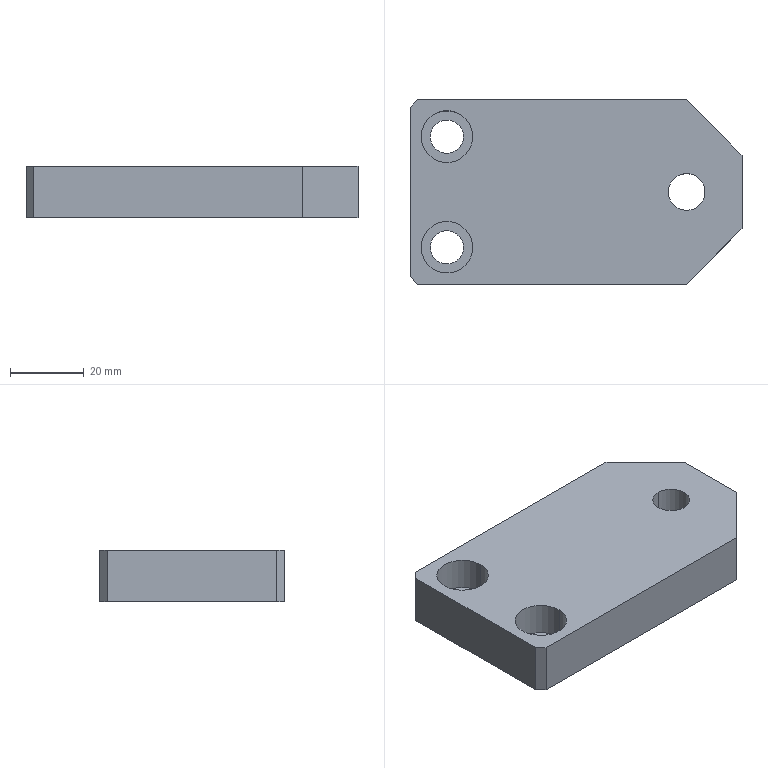Part | STEP file | J454-EBZ05-29-00-Part-1 | 1 solid | 22 faces | box 90 x 50 x 14 mm | volume 55287 mm3 | plane 12 | cylinder 10 | commonest cylinder face diameters 9 x4 14 x4 10 x2
STEP:
#1=CARTESIAN_POINT('',(14.5,40.,-2.));
#2=VERTEX_POINT('',#1);
#3=CARTESIAN_POINT('',(5.5,40.,-2.));
#4=VERTEX_POINT('',#3);
#5=CARTESIAN_POINT('',(10.,40.,-2.));
#6=DIRECTION('',(0.,0.,1.));
#7=DIRECTION('',(-1.,0.,0.));
#8=AXIS2_PLACEMENT_3D('',#5,#6,#7);
#9=CIRCLE('',#8,4.5);
#10=EDGE_CURVE('',#2,#4,#9,.T.);
#11=ORIENTED_EDGE('',*,*,#10,.F.);
#12=CARTESIAN_POINT('',(14.5,40.,3.));
#13=VERTEX_POINT('',#12);
#14=CARTESIAN_POINT('',(14.5,40.,12.));
#15=DIRECTION('',(0.,0.,1.));
#16=VECTOR('',#15,1000.);
#17=LINE('',#14,#16);
#18=EDGE_CURVE('',#2,#13,#17,.T.);
#19=ORIENTED_EDGE('',*,*,#18,.T.);
#20=CARTESIAN_POINT('',(5.5,40.,3.));
#21=VERTEX_POINT('',#20);
#22=CARTESIAN_POINT('',(10.,40.,3.));
#23=DIRECTION('',(0.,0.,1.));
#24=DIRECTION('',(-1.,0.,0.));
#25=AXIS2_PLACEMENT_3D('',#22,#23,#24);
#26=CIRCLE('',#25,4.5);
#27=EDGE_CURVE('',#13,#21,#26,.T.);
#28=ORIENTED_EDGE('',*,*,#27,.T.);
#29=CARTESIAN_POINT('',(5.5,40.,12.));
#30=DIRECTION('',(0.,0.,1.));
#31=VECTOR('',#30,1000.);
#32=LINE('',#29,#31);
#33=EDGE_CURVE('',#4,#21,#32,.T.);
#34=ORIENTED_EDGE('',*,*,#33,.F.);
#35=EDGE_LOOP('',(#11,#19,#28,#34));
#36=FACE_OUTER_BOUND('',#35,.T.);
#37=CARTESIAN_POINT('',(10.,40.,12.));
#38=DIRECTION('',(0.,0.,1.));
#39=DIRECTION('',(-1.,0.,0.));
#40=AXIS2_PLACEMENT_3D('',#37,#38,#39);
#41=CYLINDRICAL_SURFACE('',#40,4.5);
#42=ADVANCED_FACE('',(#36),#41,.F.);
#43=CARTESIAN_POINT('',(17.,40.,3.));
#44=VERTEX_POINT('',#43);
#45=CARTESIAN_POINT('',(3.,40.,3.));
#46=VERTEX_POINT('',#45);
#47=CARTESIAN_POINT('',(10.,40.,3.));
#48=DIRECTION('',(0.,0.,1.));
#49=DIRECTION('',(-1.,0.,0.));
#50=AXIS2_PLACEMENT_3D('',#47,#48,#49);
#51=CIRCLE('',#50,7.);
#52=EDGE_CURVE('',#44,#46,#51,.T.);
#53=ORIENTED_EDGE('',*,*,#52,.F.);
#54=CARTESIAN_POINT('',(17.,40.,12.));
#55=VERTEX_POINT('',#54);
#56=CARTESIAN_POINT('',(17.,40.,12.));
#57=DIRECTION('',(0.,0.,1.));
#58=VECTOR('',#57,1000.);
#59=LINE('',#56,#58);
#60=EDGE_CURVE('',#44,#55,#59,.T.);
#61=ORIENTED_EDGE('',*,*,#60,.T.);
#62=CARTESIAN_POINT('',(3.,40.,12.));
#63=VERTEX_POINT('',#62);
#64=CARTESIAN_POINT('',(10.,40.,12.));
#65=DIRECTION('',(0.,0.,1.));
#66=DIRECTION('',(-1.,0.,0.));
#67=AXIS2_PLACEMENT_3D('',#64,#65,#66);
#68=CIRCLE('',#67,7.);
#69=EDGE_CURVE('',#55,#63,#68,.T.);
#70=ORIENTED_EDGE('',*,*,#69,.T.);
#71=CARTESIAN_POINT('',(3.,40.,12.));
#72=DIRECTION('',(0.,0.,1.));
#73=VECTOR('',#72,1000.);
#74=LINE('',#71,#73);
#75=EDGE_CURVE('',#46,#63,#74,.T.);
#76=ORIENTED_EDGE('',*,*,#75,.F.);
#77=EDGE_LOOP('',(#53,#61,#70,#76));
#78=FACE_OUTER_BOUND('',#77,.T.);
#79=CARTESIAN_POINT('',(10.,40.,12.));
#80=DIRECTION('',(0.,0.,1.));
#81=DIRECTION('',(-1.,0.,0.));
#82=AXIS2_PLACEMENT_3D('',#79,#80,#81);
#83=CYLINDRICAL_SURFACE('',#82,7.);
#84=ADVANCED_FACE('',(#78),#83,.F.);
#85=CARTESIAN_POINT('',(14.5,10.,-2.));
#86=VERTEX_POINT('',#85);
#87=CARTESIAN_POINT('',(5.5,10.,-2.));
#88=VERTEX_POINT('',#87);
#89=CARTESIAN_POINT('',(10.,10.,-2.));
#90=DIRECTION('',(0.,0.,1.));
#91=DIRECTION('',(-1.,0.,0.));
#92=AXIS2_PLACEMENT_3D('',#89,#90,#91);
#93=CIRCLE('',#92,4.5);
#94=EDGE_CURVE('',#86,#88,#93,.T.);
#95=ORIENTED_EDGE('',*,*,#94,.F.);
#96=CARTESIAN_POINT('',(14.5,10.,3.));
#97=VERTEX_POINT('',#96);
#98=CARTESIAN_POINT('',(14.5,10.,12.));
#99=DIRECTION('',(0.,0.,1.));
#100=VECTOR('',#99,1000.);
#101=LINE('',#98,#100);
#102=EDGE_CURVE('',#86,#97,#101,.T.);
#103=ORIENTED_EDGE('',*,*,#102,.T.);
#104=CARTESIAN_POINT('',(5.5,10.,3.));
#105=VERTEX_POINT('',#104);
#106=CARTESIAN_POINT('',(10.,10.,3.));
#107=DIRECTION('',(0.,0.,1.));
#108=DIRECTION('',(-1.,0.,0.));
#109=AXIS2_PLACEMENT_3D('',#106,#107,#108);
#110=CIRCLE('',#109,4.5);
#111=EDGE_CURVE('',#97,#105,#110,.T.);
#112=ORIENTED_EDGE('',*,*,#111,.T.);
#113=CARTESIAN_POINT('',(5.5,10.,12.));
#114=DIRECTION('',(0.,0.,1.));
#115=VECTOR('',#114,1000.);
#116=LINE('',#113,#115);
#117=EDGE_CURVE('',#88,#105,#116,.T.);
#118=ORIENTED_EDGE('',*,*,#117,.F.);
#119=EDGE_LOOP('',(#95,#103,#112,#118));
#120=FACE_OUTER_BOUND('',#119,.T.);
#121=CARTESIAN_POINT('',(10.,10.,12.));
#122=DIRECTION('',(0.,0.,1.));
#123=DIRECTION('',(-1.,0.,0.));
#124=AXIS2_PLACEMENT_3D('',#121,#122,#123);
#125=CYLINDRICAL_SURFACE('',#124,4.5);
#126=ADVANCED_FACE('',(#120),#125,.F.);
#127=CARTESIAN_POINT('',(17.,10.,3.));
#128=VERTEX_POINT('',#127);
#129=CARTESIAN_POINT('',(3.,10.,3.));
#130=VERTEX_POINT('',#129);
#131=CARTESIAN_POINT('',(10.,10.,3.));
#132=DIRECTION('',(0.,0.,1.));
#133=DIRECTION('',(-1.,0.,0.));
#134=AXIS2_PLACEMENT_3D('',#131,#132,#133);
#135=CIRCLE('',#134,7.);
#136=EDGE_CURVE('',#128,#130,#135,.T.);
#137=ORIENTED_EDGE('',*,*,#136,.F.);
#138=CARTESIAN_POINT('',(17.,10.,12.));
#139=VERTEX_POINT('',#138);
#140=CARTESIAN_POINT('',(17.,10.,12.));
#141=DIRECTION('',(0.,0.,1.));
#142=VECTOR('',#141,1000.);
#143=LINE('',#140,#142);
#144=EDGE_CURVE('',#128,#139,#143,.T.);
#145=ORIENTED_EDGE('',*,*,#144,.T.);
#146=CARTESIAN_POINT('',(3.,10.,12.));
#147=VERTEX_POINT('',#146);
#148=CARTESIAN_POINT('',(10.,10.,12.));
#149=DIRECTION('',(0.,0.,1.));
#150=DIRECTION('',(-1.,0.,0.));
#151=AXIS2_PLACEMENT_3D('',#148,#149,#150);
#152=CIRCLE('',#151,7.);
#153=EDGE_CURVE('',#139,#147,#152,.T.);
#154=ORIENTED_EDGE('',*,*,#153,.T.);
#155=CARTESIAN_POINT('',(3.,10.,12.));
#156=DIRECTION('',(0.,0.,1.));
#157=VECTOR('',#156,1000.);
#158=LINE('',#155,#157);
#159=EDGE_CURVE('',#130,#147,#158,.T.);
#160=ORIENTED_EDGE('',*,*,#159,.F.);
#161=EDGE_LOOP('',(#137,#145,#154,#160));
#162=FACE_OUTER_BOUND('',#161,.T.);
#163=CARTESIAN_POINT('',(10.,10.,12.));
#164=DIRECTION('',(0.,0.,1.));
#165=DIRECTION('',(-1.,0.,0.));
#166=AXIS2_PLACEMENT_3D('',#163,#164,#165);
#167=CYLINDRICAL_SURFACE('',#166,7.);
#168=ADVANCED_FACE('',(#162),#167,.F.);
#169=CARTESIAN_POINT('',(75.,30.,12.));
#170=VERTEX_POINT('',#169);
#171=CARTESIAN_POINT('',(75.,20.,12.));
#172=VERTEX_POINT('',#171);
#173=CARTESIAN_POINT('',(75.,25.,12.));
#174=DIRECTION('',(0.,0.,-1.));
#175=DIRECTION('',(0.,-1.,0.));
#176=AXIS2_PLACEMENT_3D('',#173,#174,#175);
#177=CIRCLE('',#176,5.);
#178=EDGE_CURVE('',#170,#172,#177,.T.);
#179=ORIENTED_EDGE('',*,*,#178,.F.);
#180=CARTESIAN_POINT('',(75.,30.,-2.));
#181=VERTEX_POINT('',#180);
#182=CARTESIAN_POINT('',(75.,30.,12.));
#183=DIRECTION('',(0.,0.,-1.));
#184=VECTOR('',#183,1000.);
#185=LINE('',#182,#184);
#186=EDGE_CURVE('',#170,#181,#185,.T.);
#187=ORIENTED_EDGE('',*,*,#186,.T.);
#188=CARTESIAN_POINT('',(75.,20.,-2.));
#189=VERTEX_POINT('',#188);
#190=CARTESIAN_POINT('',(75.,25.,-2.));
#191=DIRECTION('',(0.,0.,1.));
#192=DIRECTION('',(0.,1.,0.));
#193=AXIS2_PLACEMENT_3D('',#190,#191,#192);
#194=CIRCLE('',#193,5.);
#195=EDGE_CURVE('',#189,#181,#194,.T.);
#196=ORIENTED_EDGE('',*,*,#195,.F.);
#197=CARTESIAN_POINT('',(75.,20.,12.));
#198=DIRECTION('',(0.,0.,-1.));
#199=VECTOR('',#198,1000.);
#200=LINE('',#197,#199);
#201=EDGE_CURVE('',#172,#189,#200,.T.);
#202=ORIENTED_EDGE('',*,*,#201,.F.);
#203=EDGE_LOOP('',(#179,#187,#196,#202));
#204=FACE_OUTER_BOUND('',#203,.T.);
#205=CARTESIAN_POINT('',(75.,25.,12.));
#206=DIRECTION('',(0.,0.,-1.));
#207=DIRECTION('',(0.,-1.,0.));
#208=AXIS2_PLACEMENT_3D('',#205,#206,#207);
#209=CYLINDRICAL_SURFACE('',#208,5.);
#210=ADVANCED_FACE('',(#204),#209,.F.);
#211=CARTESIAN_POINT('',(10.,40.,12.));
#212=DIRECTION('',(0.,0.,1.));
#213=DIRECTION('',(-1.,0.,0.));
#214=AXIS2_PLACEMENT_3D('',#211,#212,#213);
#215=CIRCLE('',#214,7.);
#216=EDGE_CURVE('',#63,#55,#215,.T.);
#217=ORIENTED_EDGE('',*,*,#216,.F.);
#218=ORIENTED_EDGE('',*,*,#69,.F.);
#219=EDGE_LOOP('',(#217,#218));
#220=FACE_BOUND('',#219,.T.);
#221=CARTESIAN_POINT('',(10.,10.,12.));
#222=DIRECTION('',(0.,0.,1.));
#223=DIRECTION('',(-1.,0.,0.));
#224=AXIS2_PLACEMENT_3D('',#221,#222,#223);
#225=CIRCLE('',#224,7.);
#226=EDGE_CURVE('',#147,#139,#225,.T.);
#227=ORIENTED_EDGE('',*,*,#226,.F.);
#228=ORIENTED_EDGE('',*,*,#153,.F.);
#229=EDGE_LOOP('',(#227,#228));
#230=FACE_BOUND('',#229,.T.);
#231=CARTESIAN_POINT('',(75.,25.,12.));
#232=DIRECTION('',(0.,0.,-1.));
#233=DIRECTION('',(0.,-1.,0.));
#234=AXIS2_PLACEMENT_3D('',#231,#232,#233);
#235=CIRCLE('',#234,5.);
#236=EDGE_CURVE('',#172,#170,#235,.T.);
#237=ORIENTED_EDGE('',*,*,#236,.T.);
#238=ORIENTED_EDGE('',*,*,#178,.T.);
#239=EDGE_LOOP('',(#237,#238));
#240=FACE_BOUND('',#239,.T.);
#241=CARTESIAN_POINT('',(2.,50.,12.));
#242=VERTEX_POINT('',#241);
#243=CARTESIAN_POINT('',(75.,50.,12.));
#244=VERTEX_POINT('',#243);
#245=CARTESIAN_POINT('',(45.,50.,12.));
#246=DIRECTION('',(1.,0.,0.));
#247=VECTOR('',#246,1000.);
#248=LINE('',#245,#247);
#249=EDGE_CURVE('',#242,#244,#248,.T.);
#250=ORIENTED_EDGE('',*,*,#249,.F.);
#251=CARTESIAN_POINT('',(0.,48.,12.));
#252=VERTEX_POINT('',#251);
#253=CARTESIAN_POINT('',(11.,59.,12.));
#254=DIRECTION('',(-0.7071,-0.7071,0.));
#255=VECTOR('',#254,1000.);
#256=LINE('',#253,#255);
#257=EDGE_CURVE('',#242,#252,#256,.T.);
#258=ORIENTED_EDGE('',*,*,#257,.T.);
#259=CARTESIAN_POINT('',(0.,2.,12.));
#260=VERTEX_POINT('',#259);
#261=CARTESIAN_POINT('',(0.,25.,12.));
#262=DIRECTION('',(0.,1.,0.));
#263=VECTOR('',#262,1000.);
#264=LINE('',#261,#263);
#265=EDGE_CURVE('',#260,#252,#264,.T.);
#266=ORIENTED_EDGE('',*,*,#265,.F.);
#267=CARTESIAN_POINT('',(2.,0.,12.));
#268=VERTEX_POINT('',#267);
#269=CARTESIAN_POINT('',(11.,-9.,12.));
#270=DIRECTION('',(0.7071,-0.7071,0.));
#271=VECTOR('',#270,1000.);
#272=LINE('',#269,#271);
#273=EDGE_CURVE('',#260,#268,#272,.T.);
#274=ORIENTED_EDGE('',*,*,#273,.T.);
#275=CARTESIAN_POINT('',(75.,0.,12.));
#276=VERTEX_POINT('',#275);
#277=CARTESIAN_POINT('',(45.,0.,12.));
#278=DIRECTION('',(-1.,0.,0.));
#279=VECTOR('',#278,1000.);
#280=LINE('',#277,#279);
#281=EDGE_CURVE('',#276,#268,#280,.T.);
#282=ORIENTED_EDGE('',*,*,#281,.F.);
#283=CARTESIAN_POINT('',(90.,15.,12.));
#284=VERTEX_POINT('',#283);
#285=CARTESIAN_POINT('',(72.5,-2.5,12.));
#286=DIRECTION('',(0.7071,0.7071,0.));
#287=VECTOR('',#286,1000.);
#288=LINE('',#285,#287);
#289=EDGE_CURVE('',#276,#284,#288,.T.);
#290=ORIENTED_EDGE('',*,*,#289,.T.);
#291=CARTESIAN_POINT('',(90.,35.,12.));
#292=VERTEX_POINT('',#291);
#293=CARTESIAN_POINT('',(90.,25.,12.));
#294=DIRECTION('',(0.,-1.,0.));
#295=VECTOR('',#294,1000.);
#296=LINE('',#293,#295);
#297=EDGE_CURVE('',#292,#284,#296,.T.);
#298=ORIENTED_EDGE('',*,*,#297,.F.);
#299=CARTESIAN_POINT('',(72.5,52.5,12.));
#300=DIRECTION('',(-0.7071,0.7071,0.));
#301=VECTOR('',#300,1000.);
#302=LINE('',#299,#301);
#303=EDGE_CURVE('',#292,#244,#302,.T.);
#304=ORIENTED_EDGE('',*,*,#303,.T.);
#305=EDGE_LOOP('',(#250,#258,#266,#274,#282,#290,#298,#304));
#306=FACE_OUTER_BOUND('',#305,.T.);
#307=CARTESIAN_POINT('',(45.,25.,12.));
#308=DIRECTION('',(0.,0.,1.));
#309=DIRECTION('',(0.,1.,0.));
#310=AXIS2_PLACEMENT_3D('',#307,#308,#309);
#311=PLANE('',#310);
#312=ADVANCED_FACE('',(#220,#230,#240,#306),#311,.T.);
#313=CARTESIAN_POINT('',(90.,15.,-2.));
#314=VERTEX_POINT('',#313);
#315=CARTESIAN_POINT('',(90.,35.,-2.));
#316=VERTEX_POINT('',#315);
#317=CARTESIAN_POINT('',(90.,25.,-2.));
#318=DIRECTION('',(0.,1.,0.));
#319=VECTOR('',#318,1000.);
#320=LINE('',#317,#319);
#321=EDGE_CURVE('',#314,#316,#320,.T.);
#322=ORIENTED_EDGE('',*,*,#321,.T.);
#323=CARTESIAN_POINT('',(90.,35.,-2.));
#324=DIRECTION('',(0.,0.,1.));
#325=VECTOR('',#324,1000.);
#326=LINE('',#323,#325);
#327=EDGE_CURVE('',#316,#292,#326,.T.);
#328=ORIENTED_EDGE('',*,*,#327,.T.);
#329=ORIENTED_EDGE('',*,*,#297,.T.);
#330=CARTESIAN_POINT('',(90.,15.,-2.));
#331=DIRECTION('',(0.,0.,-1.));
#332=VECTOR('',#331,1000.);
#333=LINE('',#330,#332);
#334=EDGE_CURVE('',#284,#314,#333,.T.);
#335=ORIENTED_EDGE('',*,*,#334,.T.);
#336=EDGE_LOOP('',(#322,#328,#329,#335));
#337=FACE_OUTER_BOUND('',#336,.T.);
#338=CARTESIAN_POINT('',(90.,25.,-2.));
#339=DIRECTION('',(1.,0.,0.));
#340=DIRECTION('',(0.,0.,-1.));
#341=AXIS2_PLACEMENT_3D('',#338,#339,#340);
#342=PLANE('',#341);
#343=ADVANCED_FACE('',(#337),#342,.T.);
#344=ORIENTED_EDGE('',*,*,#281,.T.);
#345=CARTESIAN_POINT('',(2.,0.,-2.));
#346=VERTEX_POINT('',#345);
#347=CARTESIAN_POINT('',(2.,0.,-2.));
#348=DIRECTION('',(0.,0.,-1.));
#349=VECTOR('',#348,1000.);
#350=LINE('',#347,#349);
#351=EDGE_CURVE('',#268,#346,#350,.T.);
#352=ORIENTED_EDGE('',*,*,#351,.T.);
#353=CARTESIAN_POINT('',(75.,0.,-2.));
#354=VERTEX_POINT('',#353);
#355=CARTESIAN_POINT('',(45.,0.,-2.));
#356=DIRECTION('',(1.,0.,0.));
#357=VECTOR('',#356,1000.);
#358=LINE('',#355,#357);
#359=EDGE_CURVE('',#346,#354,#358,.T.);
#360=ORIENTED_EDGE('',*,*,#359,.T.);
#361=CARTESIAN_POINT('',(75.,0.,-2.));
#362=DIRECTION('',(0.,0.,1.));
#363=VECTOR('',#362,1000.);
#364=LINE('',#361,#363);
#365=EDGE_CURVE('',#354,#276,#364,.T.);
#366=ORIENTED_EDGE('',*,*,#365,.T.);
#367=EDGE_LOOP('',(#344,#352,#360,#366));
#368=FACE_OUTER_BOUND('',#367,.T.);
#369=CARTESIAN_POINT('',(45.,0.,-2.));
#370=DIRECTION('',(0.,-1.,0.));
#371=DIRECTION('',(0.,0.,1.));
#372=AXIS2_PLACEMENT_3D('',#369,#370,#371);
#373=PLANE('',#372);
#374=ADVANCED_FACE('',(#368),#373,.T.);
#375=ORIENTED_EDGE('',*,*,#265,.T.);
#376=CARTESIAN_POINT('',(0.,48.,-2.));
#377=VERTEX_POINT('',#376);
#378=CARTESIAN_POINT('',(0.,48.,-2.));
#379=DIRECTION('',(0.,0.,-1.));
#380=VECTOR('',#379,1000.);
#381=LINE('',#378,#380);
#382=EDGE_CURVE('',#252,#377,#381,.T.);
#383=ORIENTED_EDGE('',*,*,#382,.T.);
#384=CARTESIAN_POINT('',(0.,2.,-2.));
#385=VERTEX_POINT('',#384);
#386=CARTESIAN_POINT('',(0.,25.,-2.));
#387=DIRECTION('',(0.,-1.,0.));
#388=VECTOR('',#387,1000.);
#389=LINE('',#386,#388);
#390=EDGE_CURVE('',#377,#385,#389,.T.);
#391=ORIENTED_EDGE('',*,*,#390,.T.);
#392=CARTESIAN_POINT('',(0.,2.,-2.));
#393=DIRECTION('',(0.,0.,1.));
#394=VECTOR('',#393,1000.);
#395=LINE('',#392,#394);
#396=EDGE_CURVE('',#385,#260,#395,.T.);
#397=ORIENTED_EDGE('',*,*,#396,.T.);
#398=EDGE_LOOP('',(#375,#383,#391,#397));
#399=FACE_OUTER_BOUND('',#398,.T.);
#400=CARTESIAN_POINT('',(0.,25.,-2.));
#401=DIRECTION('',(-1.,0.,0.));
#402=DIRECTION('',(0.,0.,1.));
#403=AXIS2_PLACEMENT_3D('',#400,#401,#402);
#404=PLANE('',#403);
#405=ADVANCED_FACE('',(#399),#404,.T.);
#406=CARTESIAN_POINT('',(10.,40.,-2.));
#407=DIRECTION('',(0.,0.,1.));
#408=DIRECTION('',(-1.,0.,0.));
#409=AXIS2_PLACEMENT_3D('',#406,#407,#408);
#410=CIRCLE('',#409,4.5);
#411=EDGE_CURVE('',#4,#2,#410,.T.);
#412=ORIENTED_EDGE('',*,*,#411,.T.);
#413=ORIENTED_EDGE('',*,*,#10,.T.);
#414=EDGE_LOOP('',(#412,#413));
#415=FACE_BOUND('',#414,.T.);
#416=CARTESIAN_POINT('',(10.,10.,-2.));
#417=DIRECTION('',(0.,0.,1.));
#418=DIRECTION('',(-1.,0.,0.));
#419=AXIS2_PLACEMENT_3D('',#416,#417,#418);
#420=CIRCLE('',#419,4.5);
#421=EDGE_CURVE('',#88,#86,#420,.T.);
#422=ORIENTED_EDGE('',*,*,#421,.T.);
#423=ORIENTED_EDGE('',*,*,#94,.T.);
#424=EDGE_LOOP('',(#422,#423));
#425=FACE_BOUND('',#424,.T.);
#426=ORIENTED_EDGE('',*,*,#195,.T.);
#427=CARTESIAN_POINT('',(75.,25.,-2.));
#428=DIRECTION('',(0.,0.,1.));
#429=DIRECTION('',(0.,1.,0.));
#430=AXIS2_PLACEMENT_3D('',#427,#428,#429);
#431=CIRCLE('',#430,5.);
#432=EDGE_CURVE('',#181,#189,#431,.T.);
#433=ORIENTED_EDGE('',*,*,#432,.T.);
#434=EDGE_LOOP('',(#426,#433));
#435=FACE_BOUND('',#434,.T.);
#436=ORIENTED_EDGE('',*,*,#390,.F.);
#437=CARTESIAN_POINT('',(2.,50.,-2.));
#438=VERTEX_POINT('',#437);
#439=CARTESIAN_POINT('',(11.,59.,-2.));
#440=DIRECTION('',(0.7071,0.7071,0.));
#441=VECTOR('',#440,1000.);
#442=LINE('',#439,#441);
#443=EDGE_CURVE('',#377,#438,#442,.T.);
#444=ORIENTED_EDGE('',*,*,#443,.T.);
#445=CARTESIAN_POINT('',(75.,50.,-2.));
#446=VERTEX_POINT('',#445);
#447=CARTESIAN_POINT('',(45.,50.,-2.));
#448=DIRECTION('',(-1.,0.,0.));
#449=VECTOR('',#448,1000.);
#450=LINE('',#447,#449);
#451=EDGE_CURVE('',#446,#438,#450,.T.);
#452=ORIENTED_EDGE('',*,*,#451,.F.);
#453=CARTESIAN_POINT('',(72.5,52.5,-2.));
#454=DIRECTION('',(0.7071,-0.7071,0.));
#455=VECTOR('',#454,1000.);
#456=LINE('',#453,#455);
#457=EDGE_CURVE('',#446,#316,#456,.T.);
#458=ORIENTED_EDGE('',*,*,#457,.T.);
#459=ORIENTED_EDGE('',*,*,#321,.F.);
#460=CARTESIAN_POINT('',(72.5,-2.5,-2.));
#461=DIRECTION('',(-0.7071,-0.7071,0.));
#462=VECTOR('',#461,1000.);
#463=LINE('',#460,#462);
#464=EDGE_CURVE('',#314,#354,#463,.T.);
#465=ORIENTED_EDGE('',*,*,#464,.T.);
#466=ORIENTED_EDGE('',*,*,#359,.F.);
#467=CARTESIAN_POINT('',(11.,-9.,-2.));
#468=DIRECTION('',(-0.7071,0.7071,0.));
#469=VECTOR('',#468,1000.);
#470=LINE('',#467,#469);
#471=EDGE_CURVE('',#346,#385,#470,.T.);
#472=ORIENTED_EDGE('',*,*,#471,.T.);
#473=EDGE_LOOP('',(#436,#444,#452,#458,#459,#465,#466,#472));
#474=FACE_OUTER_BOUND('',#473,.T.);
#475=CARTESIAN_POINT('',(45.,25.,-2.));
#476=DIRECTION('',(0.,0.,-1.));
#477=DIRECTION('',(0.,-1.,0.));
#478=AXIS2_PLACEMENT_3D('',#475,#476,#477);
#479=PLANE('',#478);
#480=ADVANCED_FACE('',(#415,#425,#435,#474),#479,.T.);
#481=ORIENTED_EDGE('',*,*,#451,.T.);
#482=CARTESIAN_POINT('',(2.,50.,-2.));
#483=DIRECTION('',(0.,0.,1.));
#484=VECTOR('',#483,1000.);
#485=LINE('',#482,#484);
#486=EDGE_CURVE('',#438,#242,#485,.T.);
#487=ORIENTED_EDGE('',*,*,#486,.T.);
#488=ORIENTED_EDGE('',*,*,#249,.T.);
#489=CARTESIAN_POINT('',(75.,50.,-2.));
#490=DIRECTION('',(0.,0.,-1.));
#491=VECTOR('',#490,1000.);
#492=LINE('',#489,#491);
#493=EDGE_CURVE('',#244,#446,#492,.T.);
#494=ORIENTED_EDGE('',*,*,#493,.T.);
#495=EDGE_LOOP('',(#481,#487,#488,#494));
#496=FACE_OUTER_BOUND('',#495,.T.);
#497=CARTESIAN_POINT('',(45.,50.,-2.));
#498=DIRECTION('',(0.,1.,0.));
#499=DIRECTION('',(0.,0.,-1.));
#500=AXIS2_PLACEMENT_3D('',#497,#498,#499);
#501=PLANE('',#500);
#502=ADVANCED_FACE('',(#496),#501,.T.);
#503=ORIENTED_EDGE('',*,*,#186,.F.);
#504=ORIENTED_EDGE('',*,*,#236,.F.);
#505=ORIENTED_EDGE('',*,*,#201,.T.);
#506=ORIENTED_EDGE('',*,*,#432,.F.);
#507=EDGE_LOOP('',(#503,#504,#505,#506));
#508=FACE_OUTER_BOUND('',#507,.T.);
#509=CARTESIAN_POINT('',(75.,25.,12.));
#510=DIRECTION('',(0.,0.,-1.));
#511=DIRECTION('',(0.,-1.,0.));
#512=AXIS2_PLACEMENT_3D('',#509,#510,#511);
#513=CYLINDRICAL_SURFACE('',#512,5.);
#514=ADVANCED_FACE('',(#508),#513,.F.);
#515=ORIENTED_EDGE('',*,*,#464,.F.);
#516=ORIENTED_EDGE('',*,*,#334,.F.);
#517=ORIENTED_EDGE('',*,*,#289,.F.);
#518=ORIENTED_EDGE('',*,*,#365,.F.);
#519=EDGE_LOOP('',(#515,#516,#517,#518));
#520=FACE_OUTER_BOUND('',#519,.T.);
#521=CARTESIAN_POINT('',(75.,0.,-2.));
#522=DIRECTION('',(-0.7071,0.7071,0.));
#523=DIRECTION('',(0.,0.,1.));
#524=AXIS2_PLACEMENT_3D('',#521,#522,#523);
#525=PLANE('',#524);
#526=ADVANCED_FACE('',(#520),#525,.F.);
#527=ORIENTED_EDGE('',*,*,#457,.F.);
#528=ORIENTED_EDGE('',*,*,#493,.F.);
#529=ORIENTED_EDGE('',*,*,#303,.F.);
#530=ORIENTED_EDGE('',*,*,#327,.F.);
#531=EDGE_LOOP('',(#527,#528,#529,#530));
#532=FACE_OUTER_BOUND('',#531,.T.);
#533=CARTESIAN_POINT('',(90.,35.,-2.));
#534=DIRECTION('',(-0.7071,-0.7071,0.));
#535=DIRECTION('',(0.,0.,1.));
#536=AXIS2_PLACEMENT_3D('',#533,#534,#535);
#537=PLANE('',#536);
#538=ADVANCED_FACE('',(#532),#537,.F.);
#539=ORIENTED_EDGE('',*,*,#144,.F.);
#540=CARTESIAN_POINT('',(10.,10.,3.));
#541=DIRECTION('',(0.,0.,1.));
#542=DIRECTION('',(-1.,0.,0.));
#543=AXIS2_PLACEMENT_3D('',#540,#541,#542);
#544=CIRCLE('',#543,7.);
#545=EDGE_CURVE('',#130,#128,#544,.T.);
#546=ORIENTED_EDGE('',*,*,#545,.F.);
#547=ORIENTED_EDGE('',*,*,#159,.T.);
#548=ORIENTED_EDGE('',*,*,#226,.T.);
#549=EDGE_LOOP('',(#539,#546,#547,#548));
#550=FACE_OUTER_BOUND('',#549,.T.);
#551=CARTESIAN_POINT('',(10.,10.,12.));
#552=DIRECTION('',(0.,0.,1.));
#553=DIRECTION('',(-1.,0.,0.));
#554=AXIS2_PLACEMENT_3D('',#551,#552,#553);
#555=CYLINDRICAL_SURFACE('',#554,7.);
#556=ADVANCED_FACE('',(#550),#555,.F.);
#557=CARTESIAN_POINT('',(10.,10.,3.));
#558=DIRECTION('',(0.,0.,1.));
#559=DIRECTION('',(-1.,0.,0.));
#560=AXIS2_PLACEMENT_3D('',#557,#558,#559);
#561=CIRCLE('',#560,4.5);
#562=EDGE_CURVE('',#105,#97,#561,.T.);
#563=ORIENTED_EDGE('',*,*,#562,.F.);
#564=ORIENTED_EDGE('',*,*,#111,.F.);
#565=EDGE_LOOP('',(#563,#564));
#566=FACE_BOUND('',#565,.T.);
#567=ORIENTED_EDGE('',*,*,#545,.T.);
#568=ORIENTED_EDGE('',*,*,#136,.T.);
#569=EDGE_LOOP('',(#567,#568));
#570=FACE_OUTER_BOUND('',#569,.T.);
#571=CARTESIAN_POINT('',(17.,10.,3.));
#572=DIRECTION('',(0.,0.,-1.));
#573=DIRECTION('',(1.,0.,0.));
#574=AXIS2_PLACEMENT_3D('',#571,#572,#573);
#575=PLANE('',#574);
#576=ADVANCED_FACE('',(#566,#570),#575,.F.);
#577=ORIENTED_EDGE('',*,*,#102,.F.);
#578=ORIENTED_EDGE('',*,*,#421,.F.);
#579=ORIENTED_EDGE('',*,*,#117,.T.);
#580=ORIENTED_EDGE('',*,*,#562,.T.);
#581=EDGE_LOOP('',(#577,#578,#579,#580));
#582=FACE_OUTER_BOUND('',#581,.T.);
#583=CARTESIAN_POINT('',(10.,10.,12.));
#584=DIRECTION('',(0.,0.,1.));
#585=DIRECTION('',(-1.,0.,0.));
#586=AXIS2_PLACEMENT_3D('',#583,#584,#585);
#587=CYLINDRICAL_SURFACE('',#586,4.5);
#588=ADVANCED_FACE('',(#582),#587,.F.);
#589=ORIENTED_EDGE('',*,*,#60,.F.);
#590=CARTESIAN_POINT('',(10.,40.,3.));
#591=DIRECTION('',(0.,0.,1.));
#592=DIRECTION('',(-1.,0.,0.));
#593=AXIS2_PLACEMENT_3D('',#590,#591,#592);
#594=CIRCLE('',#593,7.);
#595=EDGE_CURVE('',#46,#44,#594,.T.);
#596=ORIENTED_EDGE('',*,*,#595,.F.);
#597=ORIENTED_EDGE('',*,*,#75,.T.);
#598=ORIENTED_EDGE('',*,*,#216,.T.);
#599=EDGE_LOOP('',(#589,#596,#597,#598));
#600=FACE_OUTER_BOUND('',#599,.T.);
#601=CARTESIAN_POINT('',(10.,40.,12.));
#602=DIRECTION('',(0.,0.,1.));
#603=DIRECTION('',(-1.,0.,0.));
#604=AXIS2_PLACEMENT_3D('',#601,#602,#603);
#605=CYLINDRICAL_SURFACE('',#604,7.);
#606=ADVANCED_FACE('',(#600),#605,.F.);
#607=CARTESIAN_POINT('',(10.,40.,3.));
#608=DIRECTION('',(0.,0.,1.));
#609=DIRECTION('',(-1.,0.,0.));
#610=AXIS2_PLACEMENT_3D('',#607,#608,#609);
#611=CIRCLE('',#610,4.5);
#612=EDGE_CURVE('',#21,#13,#611,.T.);
#613=ORIENTED_EDGE('',*,*,#612,.F.);
#614=ORIENTED_EDGE('',*,*,#27,.F.);
#615=EDGE_LOOP('',(#613,#614));
#616=FACE_BOUND('',#615,.T.);
#617=ORIENTED_EDGE('',*,*,#595,.T.);
#618=ORIENTED_EDGE('',*,*,#52,.T.);
#619=EDGE_LOOP('',(#617,#618));
#620=FACE_OUTER_BOUND('',#619,.T.);
#621=CARTESIAN_POINT('',(17.,40.,3.));
#622=DIRECTION('',(0.,0.,-1.));
#623=DIRECTION('',(1.,0.,0.));
#624=AXIS2_PLACEMENT_3D('',#621,#622,#623);
#625=PLANE('',#624);
#626=ADVANCED_FACE('',(#616,#620),#625,.F.);
#627=ORIENTED_EDGE('',*,*,#18,.F.);
#628=ORIENTED_EDGE('',*,*,#411,.F.);
#629=ORIENTED_EDGE('',*,*,#33,.T.);
#630=ORIENTED_EDGE('',*,*,#612,.T.);
#631=EDGE_LOOP('',(#627,#628,#629,#630));
#632=FACE_OUTER_BOUND('',#631,.T.);
#633=CARTESIAN_POINT('',(10.,40.,12.));
#634=DIRECTION('',(0.,0.,1.));
#635=DIRECTION('',(-1.,0.,0.));
#636=AXIS2_PLACEMENT_3D('',#633,#634,#635);
#637=CYLINDRICAL_SURFACE('',#636,4.5);
#638=ADVANCED_FACE('',(#632),#637,.F.);
#639=ORIENTED_EDGE('',*,*,#471,.F.);
#640=ORIENTED_EDGE('',*,*,#351,.F.);
#641=ORIENTED_EDGE('',*,*,#273,.F.);
#642=ORIENTED_EDGE('',*,*,#396,.F.);
#643=EDGE_LOOP('',(#639,#640,#641,#642));
#644=FACE_OUTER_BOUND('',#643,.T.);
#645=CARTESIAN_POINT('',(0.,2.,-2.));
#646=DIRECTION('',(0.7071,0.7071,0.));
#647=DIRECTION('',(0.,0.,1.));
#648=AXIS2_PLACEMENT_3D('',#645,#646,#647);
#649=PLANE('',#648);
#650=ADVANCED_FACE('',(#644),#649,.F.);
#651=ORIENTED_EDGE('',*,*,#443,.F.);
#652=ORIENTED_EDGE('',*,*,#382,.F.);
#653=ORIENTED_EDGE('',*,*,#257,.F.);
#654=ORIENTED_EDGE('',*,*,#486,.F.);
#655=EDGE_LOOP('',(#651,#652,#653,#654));
#656=FACE_OUTER_BOUND('',#655,.T.);
#657=CARTESIAN_POINT('',(2.,50.,-2.));
#658=DIRECTION('',(0.7071,-0.7071,0.));
#659=DIRECTION('',(0.,0.,1.));
#660=AXIS2_PLACEMENT_3D('',#657,#658,#659);
#661=PLANE('',#660);
#662=ADVANCED_FACE('',(#656),#661,.F.);
#663=CLOSED_SHELL('',(#42,#84,#126,#168,#210,#312,#343,#374,#405,#480,#502,#514,#526,#538,#556,#576,#588,#606,#626,#638,#650,#662));
#664=MANIFOLD_SOLID_BREP('',#663);
#665=CARTESIAN_POINT('',(0.,0.,0.));
#666=DIRECTION('',(0.,0.,1.));
#667=DIRECTION('',(1.,0.,0.));
#668=AXIS2_PLACEMENT_3D('',#665,#666,#667);
#669=(LENGTH_UNIT()NAMED_UNIT(*)SI_UNIT(.MILLI.,.METRE.));
#670=UNCERTAINTY_MEASURE_WITH_UNIT(LENGTH_MEASURE(0.00001),#669,'','');
#671=(NAMED_UNIT(*)PLANE_ANGLE_UNIT()SI_UNIT($,.RADIAN.));
#672=(NAMED_UNIT(*)SI_UNIT($,.STERADIAN.)SOLID_ANGLE_UNIT());
#673=(GEOMETRIC_REPRESENTATION_CONTEXT(3)GLOBAL_UNCERTAINTY_ASSIGNED_CONTEXT((#670))GLOBAL_UNIT_ASSIGNED_CONTEXT((#669,#671,#672))REPRESENTATION_CONTEXT('',''));
#674=ADVANCED_BREP_SHAPE_REPRESENTATION('',(#664,#668),#673);